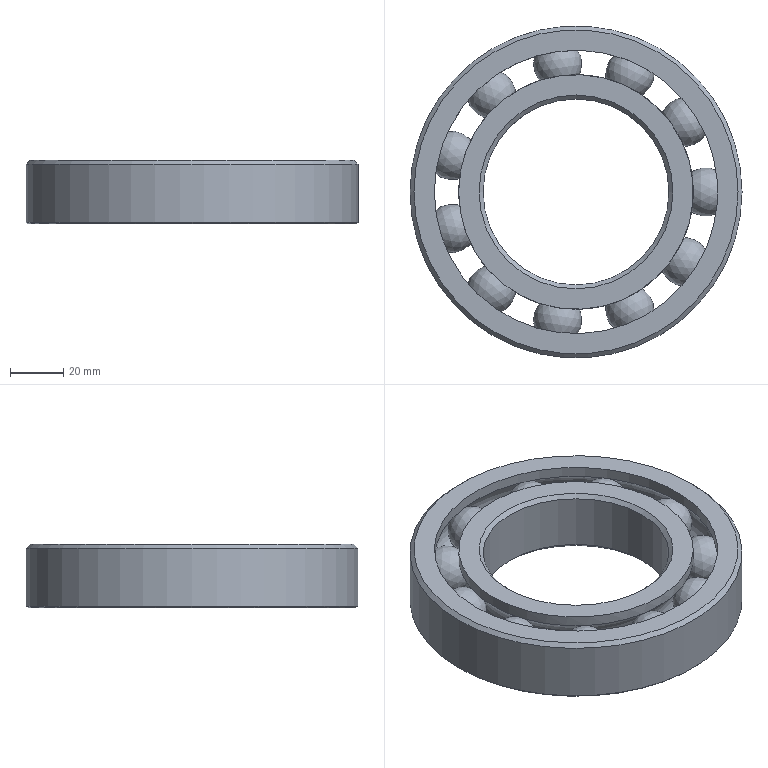Part | NX | 13 solids | 27 faces | box 125 x 125 x 24 mm | volume 136380 mm3 | sphere 11 | cylinder 5 | cone 5 | plane 4 | torus 2 | commonest cylinder face diameters 88.335 x2 70 x1 106.665 x1 125 x1
STEP:
#1=CARTESIAN_POINT('',(20.251,-44.345,2.835));
#2=VERTEX_POINT('',#1);
#3=VERTEX_LOOP('',#2);
#4=FACE_BOUND('',#3,.T.);
#5=CARTESIAN_POINT('',(20.251,-44.345,12.));
#6=DIRECTION('',(0.4154,-0.9096,0.));
#7=DIRECTION('',(0.,0.,-1.));
#8=AXIS2_PLACEMENT_3D('',#5,#6,#7);
#9=SPHERICAL_SURFACE('',#8,9.165);
#10=ADVANCED_FACE('',(#4),#9,.T.);
#11=CLOSED_SHELL('',(#10));
#12=MANIFOLD_SOLID_BREP('',#11);
#13=CARTESIAN_POINT('',(44.167,0.,4.063));
#14=VERTEX_POINT('',#13);
#15=CARTESIAN_POINT('',(0.,0.,4.063));
#16=DIRECTION('',(0.,0.,1.));
#17=DIRECTION('',(1.,0.,0.));
#18=AXIS2_PLACEMENT_3D('',#15,#16,#17);
#19=CIRCLE('',#18,44.167);
#20=EDGE_CURVE('',#14,#14,#19,.T.);
#21=ORIENTED_EDGE('',*,*,#20,.F.);
#22=EDGE_LOOP('',(#21));
#23=FACE_BOUND('',#22,.T.);
#24=CARTESIAN_POINT('',(-44.167,0.,0.));
#25=VERTEX_POINT('',#24);
#26=CARTESIAN_POINT('',(0.,0.,0.));
#27=DIRECTION('',(0.,0.,-1.));
#28=DIRECTION('',(-1.,0.,0.));
#29=AXIS2_PLACEMENT_3D('',#26,#27,#28);
#30=CIRCLE('',#29,44.167);
#31=EDGE_CURVE('',#25,#25,#30,.T.);
#32=ORIENTED_EDGE('',*,*,#31,.F.);
#33=EDGE_LOOP('',(#32));
#34=FACE_BOUND('',#33,.T.);
#35=CARTESIAN_POINT('',(0.,0.,0.));
#36=DIRECTION('',(0.,0.,-1.));
#37=DIRECTION('',(1.,0.,0.));
#38=AXIS2_PLACEMENT_3D('',#35,#36,#37);
#39=CYLINDRICAL_SURFACE('',#38,44.167);
#40=ADVANCED_FACE('',(#23,#34),#39,.T.);
#41=CARTESIAN_POINT('',(-35.,0.,1.5));
#42=VERTEX_POINT('',#41);
#43=CARTESIAN_POINT('',(0.,0.,1.5));
#44=DIRECTION('',(0.,0.,-1.));
#45=DIRECTION('',(-1.,0.,0.));
#46=AXIS2_PLACEMENT_3D('',#43,#44,#45);
#47=CIRCLE('',#46,35.);
#48=EDGE_CURVE('',#42,#42,#47,.T.);
#49=ORIENTED_EDGE('',*,*,#48,.T.);
#50=EDGE_LOOP('',(#49));
#51=FACE_BOUND('',#50,.T.);
#52=CARTESIAN_POINT('',(35.,0.,22.5));
#53=VERTEX_POINT('',#52);
#54=CARTESIAN_POINT('',(0.,0.,22.5));
#55=DIRECTION('',(0.,0.,1.));
#56=DIRECTION('',(1.,0.,0.));
#57=AXIS2_PLACEMENT_3D('',#54,#55,#56);
#58=CIRCLE('',#57,35.);
#59=EDGE_CURVE('',#53,#53,#58,.T.);
#60=ORIENTED_EDGE('',*,*,#59,.T.);
#61=EDGE_LOOP('',(#60));
#62=FACE_BOUND('',#61,.T.);
#63=CARTESIAN_POINT('',(0.,0.,0.));
#64=DIRECTION('',(0.,0.,-1.));
#65=DIRECTION('',(1.,0.,0.));
#66=AXIS2_PLACEMENT_3D('',#63,#64,#65);
#67=CYLINDRICAL_SURFACE('',#66,35.);
#68=ADVANCED_FACE('',(#51,#62),#67,.F.);
#69=CARTESIAN_POINT('',(-36.5,0.,0.));
#70=VERTEX_POINT('',#69);
#71=CARTESIAN_POINT('',(0.,0.,0.));
#72=DIRECTION('',(0.,0.,1.));
#73=DIRECTION('',(-1.,0.,0.));
#74=AXIS2_PLACEMENT_3D('',#71,#72,#73);
#75=CIRCLE('',#74,36.5);
#76=EDGE_CURVE('',#70,#70,#75,.T.);
#77=ORIENTED_EDGE('',*,*,#76,.T.);
#78=EDGE_LOOP('',(#77));
#79=FACE_BOUND('',#78,.T.);
#80=ORIENTED_EDGE('',*,*,#31,.T.);
#81=EDGE_LOOP('',(#80));
#82=FACE_BOUND('',#81,.T.);
#83=CARTESIAN_POINT('',(35.,0.,0.));
#84=DIRECTION('',(0.,0.,-1.));
#85=DIRECTION('',(1.,0.,0.));
#86=AXIS2_PLACEMENT_3D('',#83,#84,#85);
#87=PLANE('',#86);
#88=ADVANCED_FACE('',(#79,#82),#87,.T.);
#89=CARTESIAN_POINT('',(-44.167,0.,19.937));
#90=VERTEX_POINT('',#89);
#91=CARTESIAN_POINT('',(0.,0.,19.937));
#92=DIRECTION('',(0.,0.,-1.));
#93=DIRECTION('',(-1.,0.,0.));
#94=AXIS2_PLACEMENT_3D('',#91,#92,#93);
#95=CIRCLE('',#94,44.167);
#96=EDGE_CURVE('',#90,#90,#95,.T.);
#97=ORIENTED_EDGE('',*,*,#96,.F.);
#98=EDGE_LOOP('',(#97));
#99=FACE_BOUND('',#98,.T.);
#100=CARTESIAN_POINT('',(-44.167,0.,24.));
#101=VERTEX_POINT('',#100);
#102=CARTESIAN_POINT('',(0.,0.,24.));
#103=DIRECTION('',(0.,0.,-1.));
#104=DIRECTION('',(-1.,0.,0.));
#105=AXIS2_PLACEMENT_3D('',#102,#103,#104);
#106=CIRCLE('',#105,44.167);
#107=EDGE_CURVE('',#101,#101,#106,.T.);
#108=ORIENTED_EDGE('',*,*,#107,.T.);
#109=EDGE_LOOP('',(#108));
#110=FACE_BOUND('',#109,.T.);
#111=CARTESIAN_POINT('',(0.,0.,0.));
#112=DIRECTION('',(0.,0.,-1.));
#113=DIRECTION('',(1.,0.,0.));
#114=AXIS2_PLACEMENT_3D('',#111,#112,#113);
#115=CYLINDRICAL_SURFACE('',#114,44.167);
#116=ADVANCED_FACE('',(#99,#110),#115,.T.);
#117=CARTESIAN_POINT('',(36.5,0.,24.));
#118=VERTEX_POINT('',#117);
#119=CARTESIAN_POINT('',(0.,0.,24.));
#120=DIRECTION('',(0.,0.,-1.));
#121=DIRECTION('',(1.,0.,0.));
#122=AXIS2_PLACEMENT_3D('',#119,#120,#121);
#123=CIRCLE('',#122,36.5);
#124=EDGE_CURVE('',#118,#118,#123,.T.);
#125=ORIENTED_EDGE('',*,*,#124,.T.);
#126=EDGE_LOOP('',(#125));
#127=FACE_BOUND('',#126,.T.);
#128=ORIENTED_EDGE('',*,*,#107,.F.);
#129=EDGE_LOOP('',(#128));
#130=FACE_BOUND('',#129,.T.);
#131=CARTESIAN_POINT('',(44.167,0.,24.));
#132=DIRECTION('',(0.,0.,1.));
#133=DIRECTION('',(-1.,0.,0.));
#134=AXIS2_PLACEMENT_3D('',#131,#132,#133);
#135=PLANE('',#134);
#136=ADVANCED_FACE('',(#127,#130),#135,.T.);
#137=ORIENTED_EDGE('',*,*,#20,.T.);
#138=EDGE_LOOP('',(#137));
#139=FACE_BOUND('',#138,.T.);
#140=ORIENTED_EDGE('',*,*,#96,.T.);
#141=EDGE_LOOP('',(#140));
#142=FACE_BOUND('',#141,.T.);
#143=CARTESIAN_POINT('',(0.,0.,12.));
#144=DIRECTION('',(0.,0.,-1.));
#145=DIRECTION('',(1.,0.,0.));
#146=AXIS2_PLACEMENT_3D('',#143,#144,#145);
#147=TOROIDAL_SURFACE('',#146,48.75,9.165);
#148=ADVANCED_FACE('',(#139,#142),#147,.F.);
#149=ORIENTED_EDGE('',*,*,#76,.F.);
#150=EDGE_LOOP('',(#149));
#151=FACE_BOUND('',#150,.T.);
#152=ORIENTED_EDGE('',*,*,#48,.F.);
#153=EDGE_LOOP('',(#152));
#154=FACE_BOUND('',#153,.T.);
#155=CARTESIAN_POINT('',(0.,0.,1.5));
#156=DIRECTION('',(0.,0.,-1.));
#157=DIRECTION('',(1.,0.,0.));
#158=AXIS2_PLACEMENT_3D('',#155,#156,#157);
#159=CONICAL_SURFACE('',#158,35.,45.);
#160=ADVANCED_FACE('',(#151,#154),#159,.F.);
#161=ORIENTED_EDGE('',*,*,#59,.F.);
#162=EDGE_LOOP('',(#161));
#163=FACE_BOUND('',#162,.T.);
#164=ORIENTED_EDGE('',*,*,#124,.F.);
#165=EDGE_LOOP('',(#164));
#166=FACE_BOUND('',#165,.T.);
#167=CARTESIAN_POINT('',(0.,0.,24.));
#168=DIRECTION('',(0.,0.,1.));
#169=DIRECTION('',(-1.,0.,0.));
#170=AXIS2_PLACEMENT_3D('',#167,#168,#169);
#171=CONICAL_SURFACE('',#170,36.5,45.);
#172=ADVANCED_FACE('',(#163,#166),#171,.F.);
#173=CLOSED_SHELL('',(#40,#68,#88,#116,#136,#148,#160,#172));
#174=MANIFOLD_SOLID_BREP('',#173);
#175=CARTESIAN_POINT('',(-46.775,-13.734,2.835));
#176=VERTEX_POINT('',#175);
#177=VERTEX_LOOP('',#176);
#178=FACE_BOUND('',#177,.T.);
#179=CARTESIAN_POINT('',(-46.775,-13.734,12.));
#180=DIRECTION('',(-0.9595,-0.2817,0.));
#181=DIRECTION('',(0.,0.,-1.));
#182=AXIS2_PLACEMENT_3D('',#179,#180,#181);
#183=SPHERICAL_SURFACE('',#182,9.165);
#184=ADVANCED_FACE('',(#178),#183,.T.);
#185=CLOSED_SHELL('',(#184));
#186=MANIFOLD_SOLID_BREP('',#185);
#187=CARTESIAN_POINT('',(-31.924,36.843,2.835));
#188=VERTEX_POINT('',#187);
#189=VERTEX_LOOP('',#188);
#190=FACE_BOUND('',#189,.T.);
#191=CARTESIAN_POINT('',(-31.924,36.843,12.));
#192=DIRECTION('',(-0.6549,0.7557,0.));
#193=DIRECTION('',(0.,0.,-1.));
#194=AXIS2_PLACEMENT_3D('',#191,#192,#193);
#195=SPHERICAL_SURFACE('',#194,9.165);
#196=ADVANCED_FACE('',(#190),#195,.T.);
#197=CLOSED_SHELL('',(#196));
#198=MANIFOLD_SOLID_BREP('',#197);
#199=CARTESIAN_POINT('',(-6.938,48.254,2.835));
#200=VERTEX_POINT('',#199);
#201=VERTEX_LOOP('',#200);
#202=FACE_BOUND('',#201,.T.);
#203=CARTESIAN_POINT('',(-6.938,48.254,12.));
#204=DIRECTION('',(-0.1423,0.9898,0.));
#205=DIRECTION('',(0.,0.,-1.));
#206=AXIS2_PLACEMENT_3D('',#203,#204,#205);
#207=SPHERICAL_SURFACE('',#206,9.165);
#208=ADVANCED_FACE('',(#202),#207,.T.);
#209=CLOSED_SHELL('',(#208));
#210=MANIFOLD_SOLID_BREP('',#209);
#211=CARTESIAN_POINT('',(41.011,-26.356,2.835));
#212=VERTEX_POINT('',#211);
#213=VERTEX_LOOP('',#212);
#214=FACE_BOUND('',#213,.T.);
#215=CARTESIAN_POINT('',(41.011,-26.356,12.));
#216=DIRECTION('',(0.8413,-0.5406,0.));
#217=DIRECTION('',(0.,0.,-1.));
#218=AXIS2_PLACEMENT_3D('',#215,#216,#217);
#219=SPHERICAL_SURFACE('',#218,9.165);
#220=ADVANCED_FACE('',(#214),#219,.T.);
#221=CLOSED_SHELL('',(#220));
#222=MANIFOLD_SOLID_BREP('',#221);
#223=CARTESIAN_POINT('',(-46.775,13.734,2.835));
#224=VERTEX_POINT('',#223);
#225=VERTEX_LOOP('',#224);
#226=FACE_BOUND('',#225,.T.);
#227=CARTESIAN_POINT('',(-46.775,13.734,12.));
#228=DIRECTION('',(-0.9595,0.2817,0.));
#229=DIRECTION('',(0.,0.,-1.));
#230=AXIS2_PLACEMENT_3D('',#227,#228,#229);
#231=SPHERICAL_SURFACE('',#230,9.165);
#232=ADVANCED_FACE('',(#226),#231,.T.);
#233=CLOSED_SHELL('',(#232));
#234=MANIFOLD_SOLID_BREP('',#233);
#235=CARTESIAN_POINT('',(-62.5,0.,0.6));
#236=VERTEX_POINT('',#235);
#237=CARTESIAN_POINT('',(0.,0.,0.6));
#238=DIRECTION('',(0.,0.,1.));
#239=DIRECTION('',(-1.,0.,0.));
#240=AXIS2_PLACEMENT_3D('',#237,#238,#239);
#241=CIRCLE('',#240,62.5);
#242=EDGE_CURVE('',#236,#236,#241,.T.);
#243=ORIENTED_EDGE('',*,*,#242,.T.);
#244=EDGE_LOOP('',(#243));
#245=FACE_BOUND('',#244,.T.);
#246=CARTESIAN_POINT('',(62.5,0.,22.5));
#247=VERTEX_POINT('',#246);
#248=CARTESIAN_POINT('',(0.,0.,22.5));
#249=DIRECTION('',(0.,0.,-1.));
#250=DIRECTION('',(1.,0.,0.));
#251=AXIS2_PLACEMENT_3D('',#248,#249,#250);
#252=CIRCLE('',#251,62.5);
#253=EDGE_CURVE('',#247,#247,#252,.T.);
#254=ORIENTED_EDGE('',*,*,#253,.T.);
#255=EDGE_LOOP('',(#254));
#256=FACE_BOUND('',#255,.T.);
#257=CARTESIAN_POINT('',(0.,0.,0.));
#258=DIRECTION('',(0.,0.,-1.));
#259=DIRECTION('',(1.,0.,0.));
#260=AXIS2_PLACEMENT_3D('',#257,#258,#259);
#261=CYLINDRICAL_SURFACE('',#260,62.5);
#262=ADVANCED_FACE('',(#245,#256),#261,.T.);
#263=CARTESIAN_POINT('',(61.,0.,24.));
#264=VERTEX_POINT('',#263);
#265=CARTESIAN_POINT('',(0.,0.,24.));
#266=DIRECTION('',(0.,0.,1.));
#267=DIRECTION('',(1.,0.,0.));
#268=AXIS2_PLACEMENT_3D('',#265,#266,#267);
#269=CIRCLE('',#268,61.);
#270=EDGE_CURVE('',#264,#264,#269,.T.);
#271=ORIENTED_EDGE('',*,*,#270,.T.);
#272=EDGE_LOOP('',(#271));
#273=FACE_BOUND('',#272,.T.);
#274=CARTESIAN_POINT('',(-53.333,0.,24.));
#275=VERTEX_POINT('',#274);
#276=CARTESIAN_POINT('',(0.,0.,24.));
#277=DIRECTION('',(0.,0.,-1.));
#278=DIRECTION('',(-1.,0.,0.));
#279=AXIS2_PLACEMENT_3D('',#276,#277,#278);
#280=CIRCLE('',#279,53.333);
#281=EDGE_CURVE('',#275,#275,#280,.T.);
#282=ORIENTED_EDGE('',*,*,#281,.T.);
#283=EDGE_LOOP('',(#282));
#284=FACE_BOUND('',#283,.T.);
#285=CARTESIAN_POINT('',(62.5,0.,24.));
#286=DIRECTION('',(0.,0.,1.));
#287=DIRECTION('',(-1.,0.,0.));
#288=AXIS2_PLACEMENT_3D('',#285,#286,#287);
#289=PLANE('',#288);
#290=ADVANCED_FACE('',(#273,#284),#289,.T.);
#291=CARTESIAN_POINT('',(-53.333,0.,19.937));
#292=VERTEX_POINT('',#291);
#293=CARTESIAN_POINT('',(0.,0.,19.937));
#294=DIRECTION('',(0.,0.,1.));
#295=DIRECTION('',(-1.,0.,0.));
#296=AXIS2_PLACEMENT_3D('',#293,#294,#295);
#297=CIRCLE('',#296,53.333);
#298=EDGE_CURVE('',#292,#292,#297,.T.);
#299=ORIENTED_EDGE('',*,*,#298,.F.);
#300=EDGE_LOOP('',(#299));
#301=FACE_BOUND('',#300,.T.);
#302=ORIENTED_EDGE('',*,*,#281,.F.);
#303=EDGE_LOOP('',(#302));
#304=FACE_BOUND('',#303,.T.);
#305=CARTESIAN_POINT('',(0.,0.,0.));
#306=DIRECTION('',(0.,0.,-1.));
#307=DIRECTION('',(1.,0.,0.));
#308=AXIS2_PLACEMENT_3D('',#305,#306,#307);
#309=CYLINDRICAL_SURFACE('',#308,53.333);
#310=ADVANCED_FACE('',(#301,#304),#309,.F.);
#311=CARTESIAN_POINT('',(-61.9,0.,0.));
#312=VERTEX_POINT('',#311);
#313=CARTESIAN_POINT('',(0.,0.,0.));
#314=DIRECTION('',(0.,0.,-1.));
#315=DIRECTION('',(-1.,0.,0.));
#316=AXIS2_PLACEMENT_3D('',#313,#314,#315);
#317=CIRCLE('',#316,61.9);
#318=EDGE_CURVE('',#312,#312,#317,.T.);
#319=ORIENTED_EDGE('',*,*,#318,.T.);
#320=EDGE_LOOP('',(#319));
#321=FACE_BOUND('',#320,.T.);
#322=CARTESIAN_POINT('',(-55.166,0.,0.));
#323=VERTEX_POINT('',#322);
#324=CARTESIAN_POINT('',(0.,0.,0.));
#325=DIRECTION('',(0.,0.,-1.));
#326=DIRECTION('',(-1.,0.,0.));
#327=AXIS2_PLACEMENT_3D('',#324,#325,#326);
#328=CIRCLE('',#327,55.166);
#329=EDGE_CURVE('',#323,#323,#328,.T.);
#330=ORIENTED_EDGE('',*,*,#329,.F.);
#331=EDGE_LOOP('',(#330));
#332=FACE_BOUND('',#331,.T.);
#333=CARTESIAN_POINT('',(53.333,0.,0.));
#334=DIRECTION('',(0.,0.,-1.));
#335=DIRECTION('',(1.,0.,0.));
#336=AXIS2_PLACEMENT_3D('',#333,#334,#335);
#337=PLANE('',#336);
#338=ADVANCED_FACE('',(#321,#332),#337,.T.);
#339=CARTESIAN_POINT('',(-53.333,0.,4.063));
#340=VERTEX_POINT('',#339);
#341=CARTESIAN_POINT('',(0.,0.,4.063));
#342=DIRECTION('',(0.,0.,-1.));
#343=DIRECTION('',(-1.,0.,0.));
#344=AXIS2_PLACEMENT_3D('',#341,#342,#343);
#345=CIRCLE('',#344,53.333);
#346=EDGE_CURVE('',#340,#340,#345,.T.);
#347=ORIENTED_EDGE('',*,*,#346,.T.);
#348=EDGE_LOOP('',(#347));
#349=FACE_BOUND('',#348,.T.);
#350=ORIENTED_EDGE('',*,*,#298,.T.);
#351=EDGE_LOOP('',(#350));
#352=FACE_BOUND('',#351,.T.);
#353=CARTESIAN_POINT('',(0.,0.,12.));
#354=DIRECTION('',(0.,0.,-1.));
#355=DIRECTION('',(1.,0.,0.));
#356=AXIS2_PLACEMENT_3D('',#353,#354,#355);
#357=TOROIDAL_SURFACE('',#356,48.75,9.165);
#358=ADVANCED_FACE('',(#349,#352),#357,.F.);
#359=ORIENTED_EDGE('',*,*,#346,.F.);
#360=EDGE_LOOP('',(#359));
#361=FACE_BOUND('',#360,.T.);
#362=ORIENTED_EDGE('',*,*,#329,.T.);
#363=EDGE_LOOP('',(#362));
#364=FACE_BOUND('',#363,.T.);
#365=CARTESIAN_POINT('',(0.,0.,0.));
#366=DIRECTION('',(0.,0.,-1.));
#367=DIRECTION('',(1.,0.,0.));
#368=AXIS2_PLACEMENT_3D('',#365,#366,#367);
#369=CONICAL_SURFACE('',#368,55.166,24.287);
#370=ADVANCED_FACE('',(#361,#364),#369,.F.);
#371=ORIENTED_EDGE('',*,*,#270,.F.);
#372=EDGE_LOOP('',(#371));
#373=FACE_BOUND('',#372,.T.);
#374=ORIENTED_EDGE('',*,*,#253,.F.);
#375=EDGE_LOOP('',(#374));
#376=FACE_BOUND('',#375,.T.);
#377=CARTESIAN_POINT('',(0.,0.,22.5));
#378=DIRECTION('',(0.,0.,-1.));
#379=DIRECTION('',(1.,0.,0.));
#380=AXIS2_PLACEMENT_3D('',#377,#378,#379);
#381=CONICAL_SURFACE('',#380,62.5,45.);
#382=ADVANCED_FACE('',(#373,#376),#381,.T.);
#383=ORIENTED_EDGE('',*,*,#242,.F.);
#384=EDGE_LOOP('',(#383));
#385=FACE_BOUND('',#384,.T.);
#386=ORIENTED_EDGE('',*,*,#318,.F.);
#387=EDGE_LOOP('',(#386));
#388=FACE_BOUND('',#387,.T.);
#389=CARTESIAN_POINT('',(0.,0.,0.));
#390=DIRECTION('',(0.,0.,1.));
#391=DIRECTION('',(-1.,0.,0.));
#392=AXIS2_PLACEMENT_3D('',#389,#390,#391);
#393=CONICAL_SURFACE('',#392,61.9,45.);
#394=ADVANCED_FACE('',(#385,#388),#393,.T.);
#395=CLOSED_SHELL('',(#262,#290,#310,#338,#358,#370,#382,#394));
#396=MANIFOLD_SOLID_BREP('',#395);
#397=CARTESIAN_POINT('',(20.251,44.345,2.835));
#398=VERTEX_POINT('',#397);
#399=VERTEX_LOOP('',#398);
#400=FACE_BOUND('',#399,.T.);
#401=CARTESIAN_POINT('',(20.251,44.345,12.));
#402=DIRECTION('',(0.4154,0.9096,0.));
#403=DIRECTION('',(0.,0.,-1.));
#404=AXIS2_PLACEMENT_3D('',#401,#402,#403);
#405=SPHERICAL_SURFACE('',#404,9.165);
#406=ADVANCED_FACE('',(#400),#405,.T.);
#407=CLOSED_SHELL('',(#406));
#408=MANIFOLD_SOLID_BREP('',#407);
#409=CARTESIAN_POINT('',(-31.924,-36.843,2.835));
#410=VERTEX_POINT('',#409);
#411=VERTEX_LOOP('',#410);
#412=FACE_BOUND('',#411,.T.);
#413=CARTESIAN_POINT('',(-31.924,-36.843,12.));
#414=DIRECTION('',(-0.6549,-0.7557,0.));
#415=DIRECTION('',(0.,0.,-1.));
#416=AXIS2_PLACEMENT_3D('',#413,#414,#415);
#417=SPHERICAL_SURFACE('',#416,9.165);
#418=ADVANCED_FACE('',(#412),#417,.T.);
#419=CLOSED_SHELL('',(#418));
#420=MANIFOLD_SOLID_BREP('',#419);
#421=CARTESIAN_POINT('',(48.75,0.,2.835));
#422=VERTEX_POINT('',#421);
#423=VERTEX_LOOP('',#422);
#424=FACE_BOUND('',#423,.T.);
#425=CARTESIAN_POINT('',(48.75,0.,12.));
#426=DIRECTION('',(1.,0.,0.));
#427=DIRECTION('',(0.,0.,-1.));
#428=AXIS2_PLACEMENT_3D('',#425,#426,#427);
#429=SPHERICAL_SURFACE('',#428,9.165);
#430=ADVANCED_FACE('',(#424),#429,.T.);
#431=CLOSED_SHELL('',(#430));
#432=MANIFOLD_SOLID_BREP('',#431);
#433=CARTESIAN_POINT('',(-6.938,-48.254,2.835));
#434=VERTEX_POINT('',#433);
#435=VERTEX_LOOP('',#434);
#436=FACE_BOUND('',#435,.T.);
#437=CARTESIAN_POINT('',(-6.938,-48.254,12.));
#438=DIRECTION('',(-0.1423,-0.9898,0.));
#439=DIRECTION('',(0.,0.,-1.));
#440=AXIS2_PLACEMENT_3D('',#437,#438,#439);
#441=SPHERICAL_SURFACE('',#440,9.165);
#442=ADVANCED_FACE('',(#436),#441,.T.);
#443=CLOSED_SHELL('',(#442));
#444=MANIFOLD_SOLID_BREP('',#443);
#445=CARTESIAN_POINT('',(41.011,26.356,2.835));
#446=VERTEX_POINT('',#445);
#447=VERTEX_LOOP('',#446);
#448=FACE_BOUND('',#447,.T.);
#449=CARTESIAN_POINT('',(41.011,26.356,12.));
#450=DIRECTION('',(0.8413,0.5406,0.));
#451=DIRECTION('',(0.,0.,-1.));
#452=AXIS2_PLACEMENT_3D('',#449,#450,#451);
#453=SPHERICAL_SURFACE('',#452,9.165);
#454=ADVANCED_FACE('',(#448),#453,.T.);
#455=CLOSED_SHELL('',(#454));
#456=MANIFOLD_SOLID_BREP('',#455);
#457=(LENGTH_UNIT()NAMED_UNIT(*)SI_UNIT(.MILLI.,.METRE.));
#458=UNCERTAINTY_MEASURE_WITH_UNIT(LENGTH_MEASURE(0.00002),#457,'','');
#459=(NAMED_UNIT(*)PLANE_ANGLE_UNIT()SI_UNIT($,.RADIAN.));
#460=PLANE_ANGLE_MEASURE_WITH_UNIT(PLANE_ANGLE_MEASURE(0.01745),#459);
#461=DIMENSIONAL_EXPONENTS(0.,0.,0.,0.,0.,0.,0.);
#462=(CONVERSION_BASED_UNIT('DEGREE',#460)NAMED_UNIT(#461)PLANE_ANGLE_UNIT());
#463=(NAMED_UNIT(*)SI_UNIT($,.STERADIAN.)SOLID_ANGLE_UNIT());
#464=(GEOMETRIC_REPRESENTATION_CONTEXT(3)GLOBAL_UNCERTAINTY_ASSIGNED_CONTEXT((#458))GLOBAL_UNIT_ASSIGNED_CONTEXT((#457,#462,#463))REPRESENTATION_CONTEXT('',''));
#465=ADVANCED_BREP_SHAPE_REPRESENTATION('',(#12,#174,#186,#198,#210,#222,#234,#396,#408,#420,#432,#444,#456),#464);